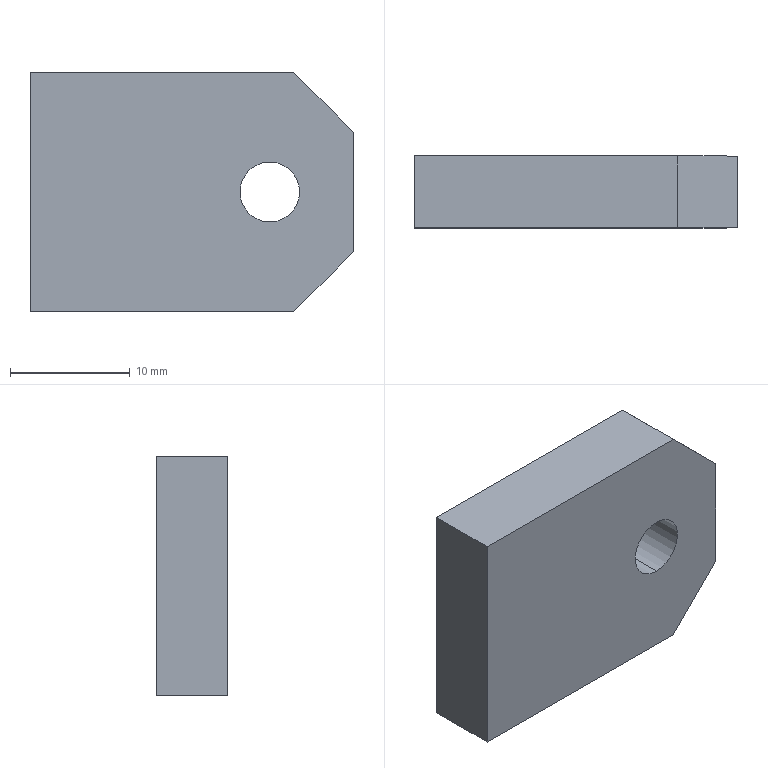Part | SolidWorks | features Chamfer 1, Extrusion 1, HoleWzd 1 | 1 solid | 10 faces | box 27 x 6 x 20 mm | volume 2972 mm3 | plane 8 | cylinder 2 | commonest cylinder face diameters 5 x2
STEP:
#1=CARTESIAN_POINT('',(6.5,-3.,7.5));
#2=VERTEX_POINT('',#1);
#3=CARTESIAN_POINT('',(6.5,-3.,12.5));
#4=VERTEX_POINT('',#3);
#5=CARTESIAN_POINT('',(6.5,-3.,10.));
#6=DIRECTION('',(0.,1.,0.));
#7=DIRECTION('',(0.,0.,1.));
#8=AXIS2_PLACEMENT_3D('',#5,#6,#7);
#9=CIRCLE('',#8,2.5);
#10=EDGE_CURVE('',#2,#4,#9,.T.);
#11=ORIENTED_EDGE('',*,*,#10,.F.);
#12=CARTESIAN_POINT('',(6.5,3.,7.5));
#13=VERTEX_POINT('',#12);
#14=CARTESIAN_POINT('',(6.5,3.,7.5));
#15=DIRECTION('',(0.,1.,0.));
#16=VECTOR('',#15,1000.);
#17=LINE('',#14,#16);
#18=EDGE_CURVE('',#2,#13,#17,.T.);
#19=ORIENTED_EDGE('',*,*,#18,.T.);
#20=CARTESIAN_POINT('',(6.5,3.,12.5));
#21=VERTEX_POINT('',#20);
#22=CARTESIAN_POINT('',(6.5,3.,10.));
#23=DIRECTION('',(0.,1.,0.));
#24=DIRECTION('',(0.,0.,1.));
#25=AXIS2_PLACEMENT_3D('',#22,#23,#24);
#26=CIRCLE('',#25,2.5);
#27=EDGE_CURVE('',#13,#21,#26,.T.);
#28=ORIENTED_EDGE('',*,*,#27,.T.);
#29=CARTESIAN_POINT('',(6.5,3.,12.5));
#30=DIRECTION('',(0.,1.,0.));
#31=VECTOR('',#30,1000.);
#32=LINE('',#29,#31);
#33=EDGE_CURVE('',#4,#21,#32,.T.);
#34=ORIENTED_EDGE('',*,*,#33,.F.);
#35=EDGE_LOOP('',(#11,#19,#28,#34));
#36=FACE_OUTER_BOUND('',#35,.T.);
#37=CARTESIAN_POINT('',(6.5,3.,10.));
#38=DIRECTION('',(0.,1.,0.));
#39=DIRECTION('',(0.,0.,1.));
#40=AXIS2_PLACEMENT_3D('',#37,#38,#39);
#41=CYLINDRICAL_SURFACE('',#40,2.5);
#42=ADVANCED_FACE('',(#36),#41,.F.);
#43=CARTESIAN_POINT('',(13.5,-3.,15.));
#44=VERTEX_POINT('',#43);
#45=CARTESIAN_POINT('',(13.5,-3.,5.));
#46=VERTEX_POINT('',#45);
#47=CARTESIAN_POINT('',(13.5,-3.,20.));
#48=DIRECTION('',(0.,0.,-1.));
#49=VECTOR('',#48,1000.);
#50=LINE('',#47,#49);
#51=EDGE_CURVE('',#44,#46,#50,.T.);
#52=ORIENTED_EDGE('',*,*,#51,.T.);
#53=CARTESIAN_POINT('',(13.5,3.,5.));
#54=VERTEX_POINT('',#53);
#55=CARTESIAN_POINT('',(13.5,3.,5.));
#56=DIRECTION('',(0.,1.,0.));
#57=VECTOR('',#56,1000.);
#58=LINE('',#55,#57);
#59=EDGE_CURVE('',#46,#54,#58,.T.);
#60=ORIENTED_EDGE('',*,*,#59,.T.);
#61=CARTESIAN_POINT('',(13.5,3.,15.));
#62=VERTEX_POINT('',#61);
#63=CARTESIAN_POINT('',(13.5,3.,20.));
#64=DIRECTION('',(0.,0.,-1.));
#65=VECTOR('',#64,1000.);
#66=LINE('',#63,#65);
#67=EDGE_CURVE('',#62,#54,#66,.T.);
#68=ORIENTED_EDGE('',*,*,#67,.F.);
#69=CARTESIAN_POINT('',(13.5,-3.,15.));
#70=DIRECTION('',(0.,-1.,0.));
#71=VECTOR('',#70,1000.);
#72=LINE('',#69,#71);
#73=EDGE_CURVE('',#62,#44,#72,.T.);
#74=ORIENTED_EDGE('',*,*,#73,.T.);
#75=EDGE_LOOP('',(#52,#60,#68,#74));
#76=FACE_OUTER_BOUND('',#75,.T.);
#77=CARTESIAN_POINT('',(13.5,3.,20.));
#78=DIRECTION('',(-1.,0.,0.));
#79=DIRECTION('',(0.,0.,1.));
#80=AXIS2_PLACEMENT_3D('',#77,#78,#79);
#81=PLANE('',#80);
#82=ADVANCED_FACE('',(#76),#81,.F.);
#83=CARTESIAN_POINT('',(6.5,3.,10.));
#84=DIRECTION('',(0.,1.,0.));
#85=DIRECTION('',(0.,0.,1.));
#86=AXIS2_PLACEMENT_3D('',#83,#84,#85);
#87=CIRCLE('',#86,2.5);
#88=EDGE_CURVE('',#21,#13,#87,.T.);
#89=ORIENTED_EDGE('',*,*,#88,.F.);
#90=ORIENTED_EDGE('',*,*,#27,.F.);
#91=EDGE_LOOP('',(#89,#90));
#92=FACE_BOUND('',#91,.T.);
#93=ORIENTED_EDGE('',*,*,#67,.T.);
#94=CARTESIAN_POINT('',(8.5,3.,0.));
#95=VERTEX_POINT('',#94);
#96=CARTESIAN_POINT('',(13.5,3.,5.));
#97=DIRECTION('',(-0.7071,0.,-0.7071));
#98=VECTOR('',#97,1000.);
#99=LINE('',#96,#98);
#100=EDGE_CURVE('',#54,#95,#99,.T.);
#101=ORIENTED_EDGE('',*,*,#100,.T.);
#102=CARTESIAN_POINT('',(-13.5,3.,0.));
#103=VERTEX_POINT('',#102);
#104=CARTESIAN_POINT('',(-13.5,3.,0.));
#105=DIRECTION('',(-1.,0.,0.));
#106=VECTOR('',#105,1000.);
#107=LINE('',#104,#106);
#108=EDGE_CURVE('',#95,#103,#107,.T.);
#109=ORIENTED_EDGE('',*,*,#108,.T.);
#110=CARTESIAN_POINT('',(-13.5,3.,20.));
#111=VERTEX_POINT('',#110);
#112=CARTESIAN_POINT('',(-13.5,3.,20.));
#113=DIRECTION('',(0.,0.,-1.));
#114=VECTOR('',#113,1000.);
#115=LINE('',#112,#114);
#116=EDGE_CURVE('',#111,#103,#115,.T.);
#117=ORIENTED_EDGE('',*,*,#116,.F.);
#118=CARTESIAN_POINT('',(8.5,3.,20.));
#119=VERTEX_POINT('',#118);
#120=CARTESIAN_POINT('',(-13.5,3.,20.));
#121=DIRECTION('',(-1.,0.,0.));
#122=VECTOR('',#121,1000.);
#123=LINE('',#120,#122);
#124=EDGE_CURVE('',#119,#111,#123,.T.);
#125=ORIENTED_EDGE('',*,*,#124,.F.);
#126=CARTESIAN_POINT('',(8.5,3.,20.));
#127=DIRECTION('',(0.7071,0.,-0.7071));
#128=VECTOR('',#127,1000.);
#129=LINE('',#126,#128);
#130=EDGE_CURVE('',#119,#62,#129,.T.);
#131=ORIENTED_EDGE('',*,*,#130,.T.);
#132=EDGE_LOOP('',(#93,#101,#109,#117,#125,#131));
#133=FACE_OUTER_BOUND('',#132,.T.);
#134=CARTESIAN_POINT('',(-13.5,3.,20.));
#135=DIRECTION('',(0.,-1.,0.));
#136=DIRECTION('',(0.,0.,-1.));
#137=AXIS2_PLACEMENT_3D('',#134,#135,#136);
#138=PLANE('',#137);
#139=ADVANCED_FACE('',(#92,#133),#138,.F.);
#140=CARTESIAN_POINT('',(-13.5,-3.,0.));
#141=VERTEX_POINT('',#140);
#142=CARTESIAN_POINT('',(-13.5,3.,0.));
#143=DIRECTION('',(0.,-1.,0.));
#144=VECTOR('',#143,1000.);
#145=LINE('',#142,#144);
#146=EDGE_CURVE('',#103,#141,#145,.T.);
#147=ORIENTED_EDGE('',*,*,#146,.T.);
#148=CARTESIAN_POINT('',(-13.5,-3.,20.));
#149=VERTEX_POINT('',#148);
#150=CARTESIAN_POINT('',(-13.5,-3.,20.));
#151=DIRECTION('',(0.,0.,-1.));
#152=VECTOR('',#151,1000.);
#153=LINE('',#150,#152);
#154=EDGE_CURVE('',#149,#141,#153,.T.);
#155=ORIENTED_EDGE('',*,*,#154,.F.);
#156=CARTESIAN_POINT('',(-13.5,3.,20.));
#157=DIRECTION('',(0.,-1.,0.));
#158=VECTOR('',#157,1000.);
#159=LINE('',#156,#158);
#160=EDGE_CURVE('',#111,#149,#159,.T.);
#161=ORIENTED_EDGE('',*,*,#160,.F.);
#162=ORIENTED_EDGE('',*,*,#116,.T.);
#163=EDGE_LOOP('',(#147,#155,#161,#162));
#164=FACE_OUTER_BOUND('',#163,.T.);
#165=CARTESIAN_POINT('',(-13.5,3.,20.));
#166=DIRECTION('',(1.,0.,0.));
#167=DIRECTION('',(0.,0.,-1.));
#168=AXIS2_PLACEMENT_3D('',#165,#166,#167);
#169=PLANE('',#168);
#170=ADVANCED_FACE('',(#164),#169,.F.);
#171=CARTESIAN_POINT('',(6.5,-3.,10.));
#172=DIRECTION('',(0.,1.,0.));
#173=DIRECTION('',(0.,0.,1.));
#174=AXIS2_PLACEMENT_3D('',#171,#172,#173);
#175=CIRCLE('',#174,2.5);
#176=EDGE_CURVE('',#4,#2,#175,.T.);
#177=ORIENTED_EDGE('',*,*,#176,.T.);
#178=ORIENTED_EDGE('',*,*,#10,.T.);
#179=EDGE_LOOP('',(#177,#178));
#180=FACE_BOUND('',#179,.T.);
#181=CARTESIAN_POINT('',(8.5,-3.,0.));
#182=VERTEX_POINT('',#181);
#183=CARTESIAN_POINT('',(-13.5,-3.,0.));
#184=DIRECTION('',(1.,0.,0.));
#185=VECTOR('',#184,1000.);
#186=LINE('',#183,#185);
#187=EDGE_CURVE('',#141,#182,#186,.T.);
#188=ORIENTED_EDGE('',*,*,#187,.T.);
#189=CARTESIAN_POINT('',(13.5,-3.,5.));
#190=DIRECTION('',(0.7071,0.,0.7071));
#191=VECTOR('',#190,1000.);
#192=LINE('',#189,#191);
#193=EDGE_CURVE('',#182,#46,#192,.T.);
#194=ORIENTED_EDGE('',*,*,#193,.T.);
#195=ORIENTED_EDGE('',*,*,#51,.F.);
#196=CARTESIAN_POINT('',(8.5,-3.,20.));
#197=VERTEX_POINT('',#196);
#198=CARTESIAN_POINT('',(8.5,-3.,20.));
#199=DIRECTION('',(-0.7071,0.,0.7071));
#200=VECTOR('',#199,1000.);
#201=LINE('',#198,#200);
#202=EDGE_CURVE('',#44,#197,#201,.T.);
#203=ORIENTED_EDGE('',*,*,#202,.T.);
#204=CARTESIAN_POINT('',(-13.5,-3.,20.));
#205=DIRECTION('',(1.,0.,0.));
#206=VECTOR('',#205,1000.);
#207=LINE('',#204,#206);
#208=EDGE_CURVE('',#149,#197,#207,.T.);
#209=ORIENTED_EDGE('',*,*,#208,.F.);
#210=ORIENTED_EDGE('',*,*,#154,.T.);
#211=EDGE_LOOP('',(#188,#194,#195,#203,#209,#210));
#212=FACE_OUTER_BOUND('',#211,.T.);
#213=CARTESIAN_POINT('',(-13.5,-3.,20.));
#214=DIRECTION('',(0.,1.,0.));
#215=DIRECTION('',(0.,0.,1.));
#216=AXIS2_PLACEMENT_3D('',#213,#214,#215);
#217=PLANE('',#216);
#218=ADVANCED_FACE('',(#180,#212),#217,.F.);
#219=ORIENTED_EDGE('',*,*,#208,.T.);
#220=CARTESIAN_POINT('',(8.5,3.,20.));
#221=DIRECTION('',(0.,1.,0.));
#222=VECTOR('',#221,1000.);
#223=LINE('',#220,#222);
#224=EDGE_CURVE('',#197,#119,#223,.T.);
#225=ORIENTED_EDGE('',*,*,#224,.T.);
#226=ORIENTED_EDGE('',*,*,#124,.T.);
#227=ORIENTED_EDGE('',*,*,#160,.T.);
#228=EDGE_LOOP('',(#219,#225,#226,#227));
#229=FACE_OUTER_BOUND('',#228,.T.);
#230=CARTESIAN_POINT('',(0.,0.,20.));
#231=DIRECTION('',(0.,0.,1.));
#232=DIRECTION('',(1.,0.,0.));
#233=AXIS2_PLACEMENT_3D('',#230,#231,#232);
#234=PLANE('',#233);
#235=ADVANCED_FACE('',(#229),#234,.T.);
#236=ORIENTED_EDGE('',*,*,#108,.F.);
#237=CARTESIAN_POINT('',(8.5,0.,0.));
#238=DIRECTION('',(0.,-1.,0.));
#239=VECTOR('',#238,1000.);
#240=LINE('',#237,#239);
#241=EDGE_CURVE('',#95,#182,#240,.T.);
#242=ORIENTED_EDGE('',*,*,#241,.T.);
#243=ORIENTED_EDGE('',*,*,#187,.F.);
#244=ORIENTED_EDGE('',*,*,#146,.F.);
#245=EDGE_LOOP('',(#236,#242,#243,#244));
#246=FACE_OUTER_BOUND('',#245,.T.);
#247=CARTESIAN_POINT('',(0.,0.,0.));
#248=DIRECTION('',(0.,0.,1.));
#249=DIRECTION('',(1.,0.,0.));
#250=AXIS2_PLACEMENT_3D('',#247,#248,#249);
#251=PLANE('',#250);
#252=ADVANCED_FACE('',(#246),#251,.F.);
#253=ORIENTED_EDGE('',*,*,#18,.F.);
#254=ORIENTED_EDGE('',*,*,#176,.F.);
#255=ORIENTED_EDGE('',*,*,#33,.T.);
#256=ORIENTED_EDGE('',*,*,#88,.T.);
#257=EDGE_LOOP('',(#253,#254,#255,#256));
#258=FACE_OUTER_BOUND('',#257,.T.);
#259=CARTESIAN_POINT('',(6.5,3.,10.));
#260=DIRECTION('',(0.,1.,0.));
#261=DIRECTION('',(0.,0.,1.));
#262=AXIS2_PLACEMENT_3D('',#259,#260,#261);
#263=CYLINDRICAL_SURFACE('',#262,2.5);
#264=ADVANCED_FACE('',(#258),#263,.F.);
#265=ORIENTED_EDGE('',*,*,#193,.F.);
#266=ORIENTED_EDGE('',*,*,#241,.F.);
#267=ORIENTED_EDGE('',*,*,#100,.F.);
#268=ORIENTED_EDGE('',*,*,#59,.F.);
#269=EDGE_LOOP('',(#265,#266,#267,#268));
#270=FACE_OUTER_BOUND('',#269,.T.);
#271=CARTESIAN_POINT('',(13.5,3.,5.));
#272=DIRECTION('',(-0.7071,0.,0.7071));
#273=DIRECTION('',(0.,1.,0.));
#274=AXIS2_PLACEMENT_3D('',#271,#272,#273);
#275=PLANE('',#274);
#276=ADVANCED_FACE('',(#270),#275,.F.);
#277=ORIENTED_EDGE('',*,*,#202,.F.);
#278=ORIENTED_EDGE('',*,*,#73,.F.);
#279=ORIENTED_EDGE('',*,*,#130,.F.);
#280=ORIENTED_EDGE('',*,*,#224,.F.);
#281=EDGE_LOOP('',(#277,#278,#279,#280));
#282=FACE_OUTER_BOUND('',#281,.T.);
#283=CARTESIAN_POINT('',(8.5,0.,20.));
#284=DIRECTION('',(0.7071,0.,0.7071));
#285=DIRECTION('',(0.,-1.,0.));
#286=AXIS2_PLACEMENT_3D('',#283,#284,#285);
#287=PLANE('',#286);
#288=ADVANCED_FACE('',(#282),#287,.T.);
#289=CLOSED_SHELL('',(#42,#82,#139,#170,#218,#235,#252,#264,#276,#288));
#290=MANIFOLD_SOLID_BREP('',#289);
#291=CARTESIAN_POINT('',(0.,0.,0.));
#292=DIRECTION('',(0.,0.,1.));
#293=DIRECTION('',(1.,0.,0.));
#294=AXIS2_PLACEMENT_3D('',#291,#292,#293);
#295=(LENGTH_UNIT()NAMED_UNIT(*)SI_UNIT(.MILLI.,.METRE.));
#296=UNCERTAINTY_MEASURE_WITH_UNIT(LENGTH_MEASURE(0.00001),#295,'','');
#297=(NAMED_UNIT(*)PLANE_ANGLE_UNIT()SI_UNIT($,.RADIAN.));
#298=(NAMED_UNIT(*)SI_UNIT($,.STERADIAN.)SOLID_ANGLE_UNIT());
#299=(GEOMETRIC_REPRESENTATION_CONTEXT(3)GLOBAL_UNCERTAINTY_ASSIGNED_CONTEXT((#296))GLOBAL_UNIT_ASSIGNED_CONTEXT((#295,#297,#298))REPRESENTATION_CONTEXT('',''));
#300=ADVANCED_BREP_SHAPE_REPRESENTATION('',(#290,#294),#299);